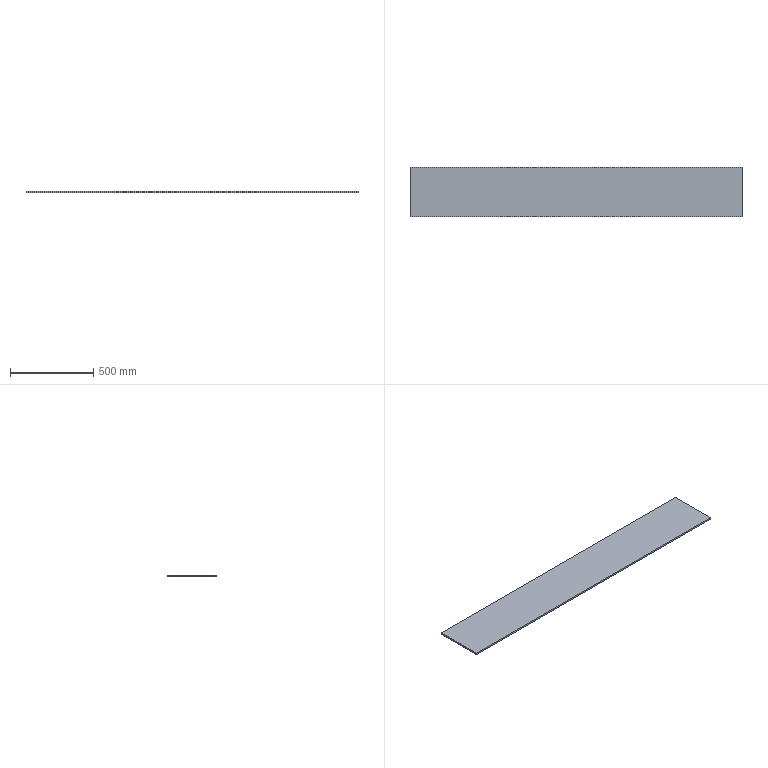Part | SolidWorks | features Extrusion 1 | 1 solid | 6 faces | box 2000 x 300 x 10 mm | volume 6000000 mm3 | plane 6
STEP:
#1=CARTESIAN_POINT('',(-1000.,150.,0.));
#2=VERTEX_POINT('',#1);
#3=CARTESIAN_POINT('',(-1000.,-150.,0.));
#4=VERTEX_POINT('',#3);
#5=CARTESIAN_POINT('',(-1000.,150.,0.));
#6=DIRECTION('',(0.,-1.,0.));
#7=VECTOR('',#6,1000.);
#8=LINE('',#5,#7);
#9=EDGE_CURVE('',#2,#4,#8,.T.);
#10=ORIENTED_EDGE('',*,*,#9,.T.);
#11=CARTESIAN_POINT('',(-1000.,-150.,10.));
#12=VERTEX_POINT('',#11);
#13=CARTESIAN_POINT('',(-1000.,-150.,10.));
#14=DIRECTION('',(0.,0.,-1.));
#15=VECTOR('',#14,1000.);
#16=LINE('',#13,#15);
#17=EDGE_CURVE('',#12,#4,#16,.T.);
#18=ORIENTED_EDGE('',*,*,#17,.F.);
#19=CARTESIAN_POINT('',(-1000.,150.,10.));
#20=VERTEX_POINT('',#19);
#21=CARTESIAN_POINT('',(-1000.,150.,10.));
#22=DIRECTION('',(0.,-1.,0.));
#23=VECTOR('',#22,1000.);
#24=LINE('',#21,#23);
#25=EDGE_CURVE('',#20,#12,#24,.T.);
#26=ORIENTED_EDGE('',*,*,#25,.F.);
#27=CARTESIAN_POINT('',(-1000.,150.,10.));
#28=DIRECTION('',(0.,0.,-1.));
#29=VECTOR('',#28,1000.);
#30=LINE('',#27,#29);
#31=EDGE_CURVE('',#20,#2,#30,.T.);
#32=ORIENTED_EDGE('',*,*,#31,.T.);
#33=EDGE_LOOP('',(#10,#18,#26,#32));
#34=FACE_OUTER_BOUND('',#33,.T.);
#35=CARTESIAN_POINT('',(-1000.,150.,10.));
#36=DIRECTION('',(1.,0.,0.));
#37=DIRECTION('',(0.,0.,-1.));
#38=AXIS2_PLACEMENT_3D('',#35,#36,#37);
#39=PLANE('',#38);
#40=ADVANCED_FACE('',(#34),#39,.F.);
#41=CARTESIAN_POINT('',(1000.,-150.,0.));
#42=VERTEX_POINT('',#41);
#43=CARTESIAN_POINT('',(1000.,-150.,0.));
#44=DIRECTION('',(1.,0.,0.));
#45=VECTOR('',#44,1000.);
#46=LINE('',#43,#45);
#47=EDGE_CURVE('',#4,#42,#46,.T.);
#48=ORIENTED_EDGE('',*,*,#47,.T.);
#49=CARTESIAN_POINT('',(1000.,-150.,10.));
#50=VERTEX_POINT('',#49);
#51=CARTESIAN_POINT('',(1000.,-150.,10.));
#52=DIRECTION('',(0.,0.,-1.));
#53=VECTOR('',#52,1000.);
#54=LINE('',#51,#53);
#55=EDGE_CURVE('',#50,#42,#54,.T.);
#56=ORIENTED_EDGE('',*,*,#55,.F.);
#57=CARTESIAN_POINT('',(1000.,-150.,10.));
#58=DIRECTION('',(1.,0.,0.));
#59=VECTOR('',#58,1000.);
#60=LINE('',#57,#59);
#61=EDGE_CURVE('',#12,#50,#60,.T.);
#62=ORIENTED_EDGE('',*,*,#61,.F.);
#63=ORIENTED_EDGE('',*,*,#17,.T.);
#64=EDGE_LOOP('',(#48,#56,#62,#63));
#65=FACE_OUTER_BOUND('',#64,.T.);
#66=CARTESIAN_POINT('',(1000.,-150.,10.));
#67=DIRECTION('',(0.,1.,0.));
#68=DIRECTION('',(-1.,0.,0.));
#69=AXIS2_PLACEMENT_3D('',#66,#67,#68);
#70=PLANE('',#69);
#71=ADVANCED_FACE('',(#65),#70,.F.);
#72=CARTESIAN_POINT('',(1000.,150.,0.));
#73=VERTEX_POINT('',#72);
#74=CARTESIAN_POINT('',(1000.,150.,0.));
#75=DIRECTION('',(0.,1.,0.));
#76=VECTOR('',#75,1000.);
#77=LINE('',#74,#76);
#78=EDGE_CURVE('',#42,#73,#77,.T.);
#79=ORIENTED_EDGE('',*,*,#78,.T.);
#80=CARTESIAN_POINT('',(1000.,150.,10.));
#81=VERTEX_POINT('',#80);
#82=CARTESIAN_POINT('',(1000.,150.,10.));
#83=DIRECTION('',(0.,0.,-1.));
#84=VECTOR('',#83,1000.);
#85=LINE('',#82,#84);
#86=EDGE_CURVE('',#81,#73,#85,.T.);
#87=ORIENTED_EDGE('',*,*,#86,.F.);
#88=CARTESIAN_POINT('',(1000.,150.,10.));
#89=DIRECTION('',(0.,1.,0.));
#90=VECTOR('',#89,1000.);
#91=LINE('',#88,#90);
#92=EDGE_CURVE('',#50,#81,#91,.T.);
#93=ORIENTED_EDGE('',*,*,#92,.F.);
#94=ORIENTED_EDGE('',*,*,#55,.T.);
#95=EDGE_LOOP('',(#79,#87,#93,#94));
#96=FACE_OUTER_BOUND('',#95,.T.);
#97=CARTESIAN_POINT('',(1000.,150.,10.));
#98=DIRECTION('',(-1.,0.,0.));
#99=DIRECTION('',(0.,0.,1.));
#100=AXIS2_PLACEMENT_3D('',#97,#98,#99);
#101=PLANE('',#100);
#102=ADVANCED_FACE('',(#96),#101,.F.);
#103=CARTESIAN_POINT('',(1000.,150.,0.));
#104=DIRECTION('',(-1.,0.,0.));
#105=VECTOR('',#104,1000.);
#106=LINE('',#103,#105);
#107=EDGE_CURVE('',#73,#2,#106,.T.);
#108=ORIENTED_EDGE('',*,*,#107,.T.);
#109=ORIENTED_EDGE('',*,*,#31,.F.);
#110=CARTESIAN_POINT('',(1000.,150.,10.));
#111=DIRECTION('',(-1.,0.,0.));
#112=VECTOR('',#111,1000.);
#113=LINE('',#110,#112);
#114=EDGE_CURVE('',#81,#20,#113,.T.);
#115=ORIENTED_EDGE('',*,*,#114,.F.);
#116=ORIENTED_EDGE('',*,*,#86,.T.);
#117=EDGE_LOOP('',(#108,#109,#115,#116));
#118=FACE_OUTER_BOUND('',#117,.T.);
#119=CARTESIAN_POINT('',(1000.,150.,10.));
#120=DIRECTION('',(0.,-1.,0.));
#121=DIRECTION('',(1.,0.,0.));
#122=AXIS2_PLACEMENT_3D('',#119,#120,#121);
#123=PLANE('',#122);
#124=ADVANCED_FACE('',(#118),#123,.F.);
#125=ORIENTED_EDGE('',*,*,#25,.T.);
#126=ORIENTED_EDGE('',*,*,#61,.T.);
#127=ORIENTED_EDGE('',*,*,#92,.T.);
#128=ORIENTED_EDGE('',*,*,#114,.T.);
#129=EDGE_LOOP('',(#125,#126,#127,#128));
#130=FACE_OUTER_BOUND('',#129,.T.);
#131=CARTESIAN_POINT('',(0.,0.,10.));
#132=DIRECTION('',(0.,0.,-1.));
#133=DIRECTION('',(-1.,0.,0.));
#134=AXIS2_PLACEMENT_3D('',#131,#132,#133);
#135=PLANE('',#134);
#136=ADVANCED_FACE('',(#130),#135,.F.);
#137=ORIENTED_EDGE('',*,*,#9,.F.);
#138=ORIENTED_EDGE('',*,*,#107,.F.);
#139=ORIENTED_EDGE('',*,*,#78,.F.);
#140=ORIENTED_EDGE('',*,*,#47,.F.);
#141=EDGE_LOOP('',(#137,#138,#139,#140));
#142=FACE_OUTER_BOUND('',#141,.T.);
#143=CARTESIAN_POINT('',(0.,0.,0.));
#144=DIRECTION('',(0.,0.,-1.));
#145=DIRECTION('',(-1.,0.,0.));
#146=AXIS2_PLACEMENT_3D('',#143,#144,#145);
#147=PLANE('',#146);
#148=ADVANCED_FACE('',(#142),#147,.T.);
#149=CLOSED_SHELL('',(#40,#71,#102,#124,#136,#148));
#150=MANIFOLD_SOLID_BREP('',#149);
#151=CARTESIAN_POINT('',(0.,0.,0.));
#152=DIRECTION('',(0.,0.,1.));
#153=DIRECTION('',(1.,0.,0.));
#154=AXIS2_PLACEMENT_3D('',#151,#152,#153);
#155=(LENGTH_UNIT()NAMED_UNIT(*)SI_UNIT(.MILLI.,.METRE.));
#156=UNCERTAINTY_MEASURE_WITH_UNIT(LENGTH_MEASURE(0.00001),#155,'','');
#157=(NAMED_UNIT(*)PLANE_ANGLE_UNIT()SI_UNIT($,.RADIAN.));
#158=(NAMED_UNIT(*)SI_UNIT($,.STERADIAN.)SOLID_ANGLE_UNIT());
#159=(GEOMETRIC_REPRESENTATION_CONTEXT(3)GLOBAL_UNCERTAINTY_ASSIGNED_CONTEXT((#156))GLOBAL_UNIT_ASSIGNED_CONTEXT((#155,#157,#158))REPRESENTATION_CONTEXT('',''));
#160=ADVANCED_BREP_SHAPE_REPRESENTATION('',(#150,#154),#159);